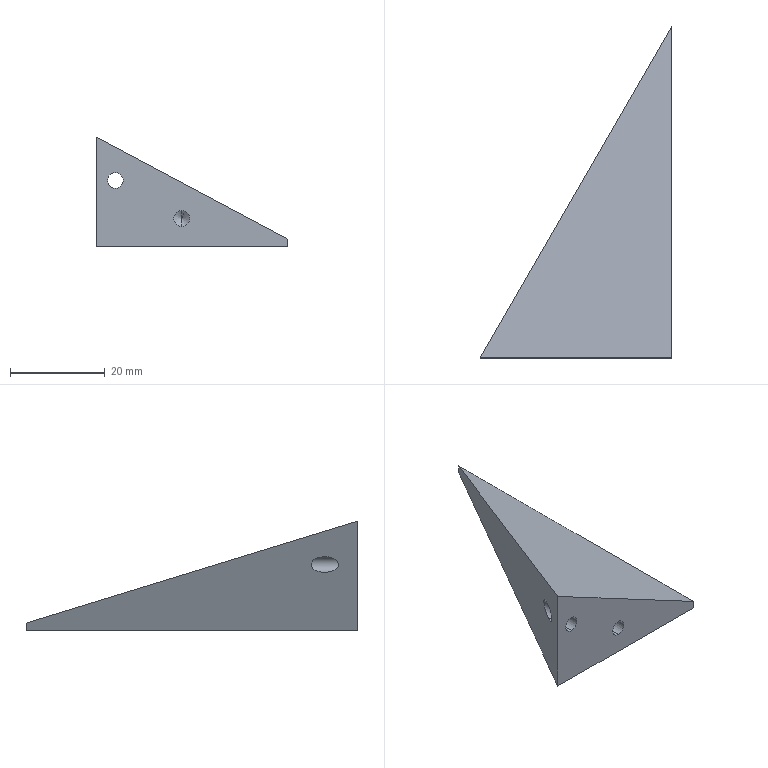Part | STEP file | GLSJ-10-26(2)_default | 1 solid | 11 faces | box 40.415 x 70 x 23.157 mm | volume 12326 mm3 | plane 5 | cylinder 4 | cone 2 | commonest cylinder face diameters 3.3 x4
STEP:
#1=CARTESIAN_POINT('',(0.,0.,0.));
#2=DIRECTION('',(0.,0.,1.));
#3=DIRECTION('',(1.,0.,0.));
#4=AXIS2_PLACEMENT_3D('',#1,#2,#3);
#5=CARTESIAN_POINT('',(-22.372,12.,-16.35));
#6=VERTEX_POINT('',#5);
#7=CARTESIAN_POINT('',(-22.372,12.,-19.65));
#8=VERTEX_POINT('',#7);
#9=CARTESIAN_POINT('',(-22.372,12.,-18.));
#10=DIRECTION('',(0.,-1.,0.));
#11=DIRECTION('',(0.,0.,-1.));
#12=AXIS2_PLACEMENT_3D('',#9,#10,#11);
#13=CIRCLE('',#12,1.65);
#14=CARTESIAN_POINT('',(-22.372,12.,-18.));
#15=DIRECTION('',(0.,-1.,0.));
#16=DIRECTION('',(0.,0.,-1.));
#17=AXIS2_PLACEMENT_3D('',#14,#15,#16);
#18=CONICAL_SURFACE('',#17,1.65,1.03);
#19=CARTESIAN_POINT('',(0.,0.));
#20=DIRECTION('',(1.,0.));
#21=VECTOR('',#20,1.);
#22=LINE('',#19,#21);
#23=(GEOMETRIC_REPRESENTATION_CONTEXT(2)PARAMETRIC_REPRESENTATION_CONTEXT()REPRESENTATION_CONTEXT('',''));
#24=DEFINITIONAL_REPRESENTATION('',(#22),#23);
#25=PCURVE('',#18,#24);
#26=CARTESIAN_POINT('',(-22.372,0.,-18.));
#27=DIRECTION('',(0.,-1.,0.));
#28=DIRECTION('',(0.,0.,1.));
#29=AXIS2_PLACEMENT_3D('',#26,#27,#28);
#30=CYLINDRICAL_SURFACE('',#29,1.65);
#31=CARTESIAN_POINT('',(-3.142,-12.));
#32=DIRECTION('',(1.,0.));
#33=VECTOR('',#32,1.);
#34=LINE('',#31,#33);
#35=(GEOMETRIC_REPRESENTATION_CONTEXT(2)PARAMETRIC_REPRESENTATION_CONTEXT()REPRESENTATION_CONTEXT('',''));
#36=DEFINITIONAL_REPRESENTATION('',(#34),#35);
#37=PCURVE('',#30,#36);
#38=SURFACE_CURVE('',#13,(#25,#37),.PCURVE_S1.);
#39=EDGE_CURVE('',#6,#8,#38,.T.);
#40=ORIENTED_EDGE('',*,*,#39,.F.);
#41=CARTESIAN_POINT('',(-22.372,12.991,-18.));
#42=VERTEX_POINT('',#41);
#43=CARTESIAN_POINT('',(-22.372,12.,-16.35));
#44=DIRECTION('',(0.,-0.515,0.8572));
#45=VECTOR('',#44,1.);
#46=LINE('',#43,#45);
#47=CARTESIAN_POINT('',(3.142,-0.9914));
#48=CARTESIAN_POINT('',(3.142,-0.9764));
#49=CARTESIAN_POINT('',(3.142,-0.9464));
#50=CARTESIAN_POINT('',(3.142,-0.9013));
#51=CARTESIAN_POINT('',(3.142,-0.8562));
#52=CARTESIAN_POINT('',(3.142,-0.8112));
#53=CARTESIAN_POINT('',(3.142,-0.7661));
#54=CARTESIAN_POINT('',(3.142,-0.721));
#55=CARTESIAN_POINT('',(3.142,-0.676));
#56=CARTESIAN_POINT('',(3.142,-0.6309));
#57=CARTESIAN_POINT('',(3.142,-0.5858));
#58=CARTESIAN_POINT('',(3.142,-0.5408));
#59=CARTESIAN_POINT('',(3.142,-0.4957));
#60=CARTESIAN_POINT('',(3.142,-0.4506));
#61=CARTESIAN_POINT('',(3.142,-0.4056));
#62=CARTESIAN_POINT('',(3.142,-0.3605));
#63=CARTESIAN_POINT('',(3.142,-0.3155));
#64=CARTESIAN_POINT('',(3.142,-0.2704));
#65=CARTESIAN_POINT('',(3.142,-0.2253));
#66=CARTESIAN_POINT('',(3.142,-0.1803));
#67=CARTESIAN_POINT('',(3.142,-0.1352));
#68=CARTESIAN_POINT('',(3.142,-0.09013));
#69=CARTESIAN_POINT('',(3.142,-0.04506));
#70=CARTESIAN_POINT('',(3.142,-0.01502));
#71=CARTESIAN_POINT('',(3.142,0.));
#72=B_SPLINE_CURVE_WITH_KNOTS('',3,(#47,#48,#49,#50,#51,#52,#53,#54,#55,#56,#57,#58,#59,#60,#61,#62,#63,#64,#65,#66,#67,#68,#69,#70,#71),.UNSPECIFIED.,.F.,.F.,(4,1,1,1,1,1,1,1,1,1,1,1,1,1,1,1,1,1,1,1,1,1,4),(-1.925,-1.837,-1.75,-1.662,-1.575,-1.487,-1.4,-1.312,-1.225,-1.137,-1.05,-0.9625,-0.875,-0.7875,-0.7,-0.6125,-0.525,-0.4375,-0.35,-0.2625,-0.175,-0.0875,0.),.QUASI_UNIFORM_KNOTS.);
#73=(GEOMETRIC_REPRESENTATION_CONTEXT(2)PARAMETRIC_REPRESENTATION_CONTEXT()REPRESENTATION_CONTEXT('',''));
#74=DEFINITIONAL_REPRESENTATION('',(#72),#73);
#75=PCURVE('',#18,#74);
#76=CARTESIAN_POINT('',(-22.372,12.,-18.));
#77=DIRECTION('',(0.,-1.,0.));
#78=DIRECTION('',(0.,0.,-1.));
#79=AXIS2_PLACEMENT_3D('',#76,#77,#78);
#80=CONICAL_SURFACE('',#79,1.65,1.03);
#81=CARTESIAN_POINT('',(3.142,-0.9914));
#82=CARTESIAN_POINT('',(3.142,-0.9764));
#83=CARTESIAN_POINT('',(3.142,-0.9464));
#84=CARTESIAN_POINT('',(3.142,-0.9013));
#85=CARTESIAN_POINT('',(3.142,-0.8562));
#86=CARTESIAN_POINT('',(3.142,-0.8112));
#87=CARTESIAN_POINT('',(3.142,-0.7661));
#88=CARTESIAN_POINT('',(3.142,-0.721));
#89=CARTESIAN_POINT('',(3.142,-0.676));
#90=CARTESIAN_POINT('',(3.142,-0.6309));
#91=CARTESIAN_POINT('',(3.142,-0.5858));
#92=CARTESIAN_POINT('',(3.142,-0.5408));
#93=CARTESIAN_POINT('',(3.142,-0.4957));
#94=CARTESIAN_POINT('',(3.142,-0.4506));
#95=CARTESIAN_POINT('',(3.142,-0.4056));
#96=CARTESIAN_POINT('',(3.142,-0.3605));
#97=CARTESIAN_POINT('',(3.142,-0.3155));
#98=CARTESIAN_POINT('',(3.142,-0.2704));
#99=CARTESIAN_POINT('',(3.142,-0.2253));
#100=CARTESIAN_POINT('',(3.142,-0.1803));
#101=CARTESIAN_POINT('',(3.142,-0.1352));
#102=CARTESIAN_POINT('',(3.142,-0.09013));
#103=CARTESIAN_POINT('',(3.142,-0.04506));
#104=CARTESIAN_POINT('',(3.142,-0.01502));
#105=CARTESIAN_POINT('',(3.142,0.));
#106=B_SPLINE_CURVE_WITH_KNOTS('',3,(#81,#82,#83,#84,#85,#86,#87,#88,#89,#90,#91,#92,#93,#94,#95,#96,#97,#98,#99,#100,#101,#102,#103,#104,#105),.UNSPECIFIED.,.F.,.F.,(4,1,1,1,1,1,1,1,1,1,1,1,1,1,1,1,1,1,1,1,1,1,4),(-1.925,-1.837,-1.75,-1.662,-1.575,-1.487,-1.4,-1.312,-1.225,-1.137,-1.05,-0.9625,-0.875,-0.7875,-0.7,-0.6125,-0.525,-0.4375,-0.35,-0.2625,-0.175,-0.0875,0.),.QUASI_UNIFORM_KNOTS.);
#107=(GEOMETRIC_REPRESENTATION_CONTEXT(2)PARAMETRIC_REPRESENTATION_CONTEXT()REPRESENTATION_CONTEXT('',''));
#108=DEFINITIONAL_REPRESENTATION('',(#106),#107);
#109=PCURVE('',#80,#108);
#110=SURFACE_CURVE('',#46,(#75,#109),.PCURVE_S1.);
#111=EDGE_CURVE('',#42,#6,#110,.T.);
#112=ORIENTED_EDGE('',*,*,#111,.F.);
#113=CARTESIAN_POINT('',(-22.372,12.,-19.65));
#114=DIRECTION('',(0.,-0.515,-0.8572));
#115=VECTOR('',#114,1.);
#116=LINE('',#113,#115);
#117=CARTESIAN_POINT('',(6.283,0.));
#118=DIRECTION('',(0.,1.));
#119=VECTOR('',#118,1.);
#120=LINE('',#117,#119);
#121=(GEOMETRIC_REPRESENTATION_CONTEXT(2)PARAMETRIC_REPRESENTATION_CONTEXT()REPRESENTATION_CONTEXT('',''));
#122=DEFINITIONAL_REPRESENTATION('',(#120),#121);
#123=PCURVE('',#18,#122);
#124=CARTESIAN_POINT('',(0.,0.));
#125=DIRECTION('',(0.,1.));
#126=VECTOR('',#125,1.);
#127=LINE('',#124,#126);
#128=(GEOMETRIC_REPRESENTATION_CONTEXT(2)PARAMETRIC_REPRESENTATION_CONTEXT()REPRESENTATION_CONTEXT('',''));
#129=DEFINITIONAL_REPRESENTATION('',(#127),#128);
#130=PCURVE('',#80,#129);
#131=SURFACE_CURVE('',#116,(#123,#130),.PCURVE_S1.);
#132=EDGE_CURVE('',#42,#8,#131,.T.);
#133=ORIENTED_EDGE('',*,*,#132,.T.);
#134=EDGE_LOOP('',(#40,#112,#133));
#135=FACE_BOUND('',#134,.F.);
#136=ADVANCED_FACE('',(#135),#18,.F.);
#137=CARTESIAN_POINT('',(-36.372,7.003,-8.35));
#138=VERTEX_POINT('',#137);
#139=CARTESIAN_POINT('',(-36.372,0.,-8.35));
#140=VERTEX_POINT('',#139);
#141=CARTESIAN_POINT('',(-36.372,0.,-8.35));
#142=DIRECTION('',(0.,-1.,0.));
#143=VECTOR('',#142,1.);
#144=LINE('',#141,#143);
#145=CARTESIAN_POINT('',(-36.372,0.,-10.));
#146=DIRECTION('',(0.,-1.,0.));
#147=DIRECTION('',(0.,0.,1.));
#148=AXIS2_PLACEMENT_3D('',#145,#146,#147);
#149=CYLINDRICAL_SURFACE('',#148,1.65);
#150=CARTESIAN_POINT('',(6.283,0.));
#151=DIRECTION('',(0.,1.));
#152=VECTOR('',#151,1.);
#153=LINE('',#150,#152);
#154=(GEOMETRIC_REPRESENTATION_CONTEXT(2)PARAMETRIC_REPRESENTATION_CONTEXT()REPRESENTATION_CONTEXT('',''));
#155=DEFINITIONAL_REPRESENTATION('',(#153),#154);
#156=PCURVE('',#149,#155);
#157=CARTESIAN_POINT('',(-36.372,0.,-10.));
#158=DIRECTION('',(0.,-1.,0.));
#159=DIRECTION('',(0.,0.,1.));
#160=AXIS2_PLACEMENT_3D('',#157,#158,#159);
#161=CYLINDRICAL_SURFACE('',#160,1.65);
#162=CARTESIAN_POINT('',(0.,0.));
#163=DIRECTION('',(0.,1.));
#164=VECTOR('',#163,1.);
#165=LINE('',#162,#164);
#166=(GEOMETRIC_REPRESENTATION_CONTEXT(2)PARAMETRIC_REPRESENTATION_CONTEXT()REPRESENTATION_CONTEXT('',''));
#167=DEFINITIONAL_REPRESENTATION('',(#165),#166);
#168=PCURVE('',#161,#167);
#169=SURFACE_CURVE('',#144,(#156,#168),.PCURVE_S1.);
#170=EDGE_CURVE('',#138,#140,#169,.T.);
#171=ORIENTED_EDGE('',*,*,#170,.T.);
#172=CARTESIAN_POINT('',(-36.372,0.,-11.65));
#173=VERTEX_POINT('',#172);
#174=CARTESIAN_POINT('',(-36.372,0.,-10.));
#175=DIRECTION('',(0.,1.,0.));
#176=DIRECTION('',(0.,0.,1.));
#177=AXIS2_PLACEMENT_3D('',#174,#175,#176);
#178=CIRCLE('',#177,1.65);
#179=CARTESIAN_POINT('',(6.283,0.));
#180=DIRECTION('',(-1.,0.));
#181=VECTOR('',#180,1.);
#182=LINE('',#179,#181);
#183=(GEOMETRIC_REPRESENTATION_CONTEXT(2)PARAMETRIC_REPRESENTATION_CONTEXT()REPRESENTATION_CONTEXT('',''));
#184=DEFINITIONAL_REPRESENTATION('',(#182),#183);
#185=PCURVE('',#149,#184);
#186=CARTESIAN_POINT('',(-40.415,0.,-24.));
#187=DIRECTION('',(0.,1.,0.));
#188=DIRECTION('',(-1.,0.,0.));
#189=AXIS2_PLACEMENT_3D('',#186,#187,#188);
#190=PLANE('',#189);
#191=CARTESIAN_POINT('',(-4.043,14.));
#192=DIRECTION('',(0.,1.));
#193=AXIS2_PLACEMENT_2D('',#191,#192);
#194=CIRCLE('',#193,1.65);
#195=(GEOMETRIC_REPRESENTATION_CONTEXT(2)PARAMETRIC_REPRESENTATION_CONTEXT()REPRESENTATION_CONTEXT('',''));
#196=DEFINITIONAL_REPRESENTATION('',(#194),#195);
#197=PCURVE('',#190,#196);
#198=SURFACE_CURVE('',#178,(#185,#197),.PCURVE_S1.);
#199=EDGE_CURVE('',#140,#173,#198,.T.);
#200=ORIENTED_EDGE('',*,*,#199,.T.);
#201=CARTESIAN_POINT('',(-36.372,7.003,-11.65));
#202=VERTEX_POINT('',#201);
#203=CARTESIAN_POINT('',(-36.372,0.,-11.65));
#204=DIRECTION('',(0.,-1.,0.));
#205=VECTOR('',#204,1.);
#206=LINE('',#203,#205);
#207=CARTESIAN_POINT('',(3.142,0.));
#208=DIRECTION('',(0.,1.));
#209=VECTOR('',#208,1.);
#210=LINE('',#207,#209);
#211=(GEOMETRIC_REPRESENTATION_CONTEXT(2)PARAMETRIC_REPRESENTATION_CONTEXT()REPRESENTATION_CONTEXT('',''));
#212=DEFINITIONAL_REPRESENTATION('',(#210),#211);
#213=PCURVE('',#149,#212);
#214=CARTESIAN_POINT('',(3.142,0.));
#215=DIRECTION('',(0.,1.));
#216=VECTOR('',#215,1.);
#217=LINE('',#214,#216);
#218=(GEOMETRIC_REPRESENTATION_CONTEXT(2)PARAMETRIC_REPRESENTATION_CONTEXT()REPRESENTATION_CONTEXT('',''));
#219=DEFINITIONAL_REPRESENTATION('',(#217),#218);
#220=PCURVE('',#161,#219);
#221=SURFACE_CURVE('',#206,(#213,#220),.PCURVE_S1.);
#222=EDGE_CURVE('',#202,#173,#221,.T.);
#223=ORIENTED_EDGE('',*,*,#222,.F.);
#224=CARTESIAN_POINT('',(-36.372,7.003,-8.35));
#225=CARTESIAN_POINT('',(-33.072,12.718,-8.35));
#226=CARTESIAN_POINT('',(-33.072,12.718,-11.65));
#227=CARTESIAN_POINT('',(-36.372,7.003,-11.65));
#228=(BOUNDED_CURVE()B_SPLINE_CURVE(3,(#224,#225,#226,#227),.UNSPECIFIED.,.F.,.F.)B_SPLINE_CURVE_WITH_KNOTS((4,4),(1.571,4.712),.PIECEWISE_BEZIER_KNOTS.)CURVE()GEOMETRIC_REPRESENTATION_ITEM()RATIONAL_B_SPLINE_CURVE((1.,0.3333,0.3333,1.))REPRESENTATION_ITEM(''));
#229=CARTESIAN_POINT('',(6.283,-7.003));
#230=CARTESIAN_POINT('',(6.253,-7.089));
#231=CARTESIAN_POINT('',(6.19,-7.27));
#232=CARTESIAN_POINT('',(6.085,-7.565));
#233=CARTESIAN_POINT('',(5.972,-7.88));
#234=CARTESIAN_POINT('',(5.848,-8.212));
#235=CARTESIAN_POINT('',(5.713,-8.551));
#236=CARTESIAN_POINT('',(5.567,-8.885));
#237=CARTESIAN_POINT('',(5.412,-9.199));
#238=CARTESIAN_POINT('',(5.246,-9.475));
#239=CARTESIAN_POINT('',(5.073,-9.69));
#240=CARTESIAN_POINT('',(4.894,-9.829));
#241=CARTESIAN_POINT('',(4.712,-9.876));
#242=CARTESIAN_POINT('',(4.531,-9.829));
#243=CARTESIAN_POINT('',(4.352,-9.69));
#244=CARTESIAN_POINT('',(4.179,-9.475));
#245=CARTESIAN_POINT('',(4.013,-9.199));
#246=CARTESIAN_POINT('',(3.857,-8.885));
#247=CARTESIAN_POINT('',(3.712,-8.551));
#248=CARTESIAN_POINT('',(3.577,-8.212));
#249=CARTESIAN_POINT('',(3.453,-7.88));
#250=CARTESIAN_POINT('',(3.339,-7.565));
#251=CARTESIAN_POINT('',(3.235,-7.27));
#252=CARTESIAN_POINT('',(3.172,-7.089));
#253=CARTESIAN_POINT('',(3.142,-7.003));
#254=B_SPLINE_CURVE_WITH_KNOTS('',3,(#229,#230,#231,#232,#233,#234,#235,#236,#237,#238,#239,#240,#241,#242,#243,#244,#245,#246,#247,#248,#249,#250,#251,#252,#253),.UNSPECIFIED.,.F.,.F.,(4,1,1,1,1,1,1,1,1,1,1,1,1,1,1,1,1,1,1,1,1,1,4),(1.571,1.714,1.856,1.999,2.142,2.285,2.428,2.57,2.713,2.856,2.999,3.142,3.284,3.427,3.57,3.713,3.856,3.998,4.141,4.284,4.427,4.57,4.712),.QUASI_UNIFORM_KNOTS.);
#255=(GEOMETRIC_REPRESENTATION_CONTEXT(2)PARAMETRIC_REPRESENTATION_CONTEXT()REPRESENTATION_CONTEXT('',''));
#256=DEFINITIONAL_REPRESENTATION('',(#254),#255);
#257=PCURVE('',#149,#256);
#258=CARTESIAN_POINT('',(0.,70.,-24.));
#259=DIRECTION('',(0.866,-0.5,0.));
#260=DIRECTION('',(0.5,0.866,0.));
#261=AXIS2_PLACEMENT_3D('',#258,#259,#260);
#262=PLANE('',#261);
#263=CARTESIAN_POINT('',(-72.743,15.65));
#264=CARTESIAN_POINT('',(-66.143,15.65));
#265=CARTESIAN_POINT('',(-66.143,12.35));
#266=CARTESIAN_POINT('',(-72.743,12.35));
#267=(BOUNDED_CURVE()B_SPLINE_CURVE(3,(#263,#264,#265,#266),.UNSPECIFIED.,.F.,.F.)B_SPLINE_CURVE_WITH_KNOTS((4,4),(1.571,4.712),.PIECEWISE_BEZIER_KNOTS.)CURVE()GEOMETRIC_REPRESENTATION_ITEM()RATIONAL_B_SPLINE_CURVE((1.,0.3333,0.3333,1.))REPRESENTATION_ITEM(''));
#268=(GEOMETRIC_REPRESENTATION_CONTEXT(2)PARAMETRIC_REPRESENTATION_CONTEXT()REPRESENTATION_CONTEXT('',''));
#269=DEFINITIONAL_REPRESENTATION('',(#267),#268);
#270=PCURVE('',#262,#269);
#271=SURFACE_CURVE('',#228,(#257,#270),.PCURVE_S1.);
#272=EDGE_CURVE('',#138,#202,#271,.T.);
#273=ORIENTED_EDGE('',*,*,#272,.F.);
#274=EDGE_LOOP('',(#171,#200,#223,#273));
#275=FACE_BOUND('',#274,.F.);
#276=ADVANCED_FACE('',(#275),#149,.F.);
#277=CARTESIAN_POINT('',(-22.372,0.,-16.35));
#278=VERTEX_POINT('',#277);
#279=CARTESIAN_POINT('',(-22.372,0.,-16.35));
#280=DIRECTION('',(0.,-1.,0.));
#281=VECTOR('',#280,1.);
#282=LINE('',#279,#281);
#283=CARTESIAN_POINT('',(-22.372,0.,-18.));
#284=DIRECTION('',(0.,-1.,0.));
#285=DIRECTION('',(0.,0.,1.));
#286=AXIS2_PLACEMENT_3D('',#283,#284,#285);
#287=CYLINDRICAL_SURFACE('',#286,1.65);
#288=CARTESIAN_POINT('',(6.283,0.));
#289=DIRECTION('',(0.,1.));
#290=VECTOR('',#289,1.);
#291=LINE('',#288,#290);
#292=(GEOMETRIC_REPRESENTATION_CONTEXT(2)PARAMETRIC_REPRESENTATION_CONTEXT()REPRESENTATION_CONTEXT('',''));
#293=DEFINITIONAL_REPRESENTATION('',(#291),#292);
#294=PCURVE('',#287,#293);
#295=CARTESIAN_POINT('',(0.,0.));
#296=DIRECTION('',(0.,1.));
#297=VECTOR('',#296,1.);
#298=LINE('',#295,#297);
#299=(GEOMETRIC_REPRESENTATION_CONTEXT(2)PARAMETRIC_REPRESENTATION_CONTEXT()REPRESENTATION_CONTEXT('',''));
#300=DEFINITIONAL_REPRESENTATION('',(#298),#299);
#301=PCURVE('',#30,#300);
#302=SURFACE_CURVE('',#282,(#294,#301),.PCURVE_S1.);
#303=EDGE_CURVE('',#6,#278,#302,.T.);
#304=ORIENTED_EDGE('',*,*,#303,.T.);
#305=CARTESIAN_POINT('',(-22.372,0.,-19.65));
#306=VERTEX_POINT('',#305);
#307=CARTESIAN_POINT('',(-22.372,0.,-18.));
#308=DIRECTION('',(0.,1.,0.));
#309=DIRECTION('',(0.,0.,1.));
#310=AXIS2_PLACEMENT_3D('',#307,#308,#309);
#311=CIRCLE('',#310,1.65);
#312=CARTESIAN_POINT('',(6.283,0.));
#313=DIRECTION('',(-1.,0.));
#314=VECTOR('',#313,1.);
#315=LINE('',#312,#314);
#316=(GEOMETRIC_REPRESENTATION_CONTEXT(2)PARAMETRIC_REPRESENTATION_CONTEXT()REPRESENTATION_CONTEXT('',''));
#317=DEFINITIONAL_REPRESENTATION('',(#315),#316);
#318=PCURVE('',#287,#317);
#319=CARTESIAN_POINT('',(-18.043,6.));
#320=DIRECTION('',(0.,1.));
#321=AXIS2_PLACEMENT_2D('',#319,#320);
#322=CIRCLE('',#321,1.65);
#323=(GEOMETRIC_REPRESENTATION_CONTEXT(2)PARAMETRIC_REPRESENTATION_CONTEXT()REPRESENTATION_CONTEXT('',''));
#324=DEFINITIONAL_REPRESENTATION('',(#322),#323);
#325=PCURVE('',#190,#324);
#326=SURFACE_CURVE('',#311,(#318,#325),.PCURVE_S1.);
#327=EDGE_CURVE('',#278,#306,#326,.T.);
#328=ORIENTED_EDGE('',*,*,#327,.T.);
#329=CARTESIAN_POINT('',(-22.372,0.,-19.65));
#330=DIRECTION('',(0.,-1.,0.));
#331=VECTOR('',#330,1.);
#332=LINE('',#329,#331);
#333=CARTESIAN_POINT('',(3.142,0.));
#334=DIRECTION('',(0.,1.));
#335=VECTOR('',#334,1.);
#336=LINE('',#333,#335);
#337=(GEOMETRIC_REPRESENTATION_CONTEXT(2)PARAMETRIC_REPRESENTATION_CONTEXT()REPRESENTATION_CONTEXT('',''));
#338=DEFINITIONAL_REPRESENTATION('',(#336),#337);
#339=PCURVE('',#287,#338);
#340=CARTESIAN_POINT('',(3.142,0.));
#341=DIRECTION('',(0.,1.));
#342=VECTOR('',#341,1.);
#343=LINE('',#340,#342);
#344=(GEOMETRIC_REPRESENTATION_CONTEXT(2)PARAMETRIC_REPRESENTATION_CONTEXT()REPRESENTATION_CONTEXT('',''));
#345=DEFINITIONAL_REPRESENTATION('',(#343),#344);
#346=PCURVE('',#30,#345);
#347=SURFACE_CURVE('',#332,(#339,#346),.PCURVE_S1.);
#348=EDGE_CURVE('',#8,#306,#347,.T.);
#349=ORIENTED_EDGE('',*,*,#348,.F.);
#350=CARTESIAN_POINT('',(-22.372,12.,-18.));
#351=DIRECTION('',(0.,-1.,0.));
#352=DIRECTION('',(0.,0.,-1.));
#353=AXIS2_PLACEMENT_3D('',#350,#351,#352);
#354=CIRCLE('',#353,1.65);
#355=CARTESIAN_POINT('',(3.142,-12.));
#356=DIRECTION('',(1.,0.));
#357=VECTOR('',#356,1.);
#358=LINE('',#355,#357);
#359=(GEOMETRIC_REPRESENTATION_CONTEXT(2)PARAMETRIC_REPRESENTATION_CONTEXT()REPRESENTATION_CONTEXT('',''));
#360=DEFINITIONAL_REPRESENTATION('',(#358),#359);
#361=PCURVE('',#287,#360);
#362=CARTESIAN_POINT('',(0.,0.));
#363=DIRECTION('',(1.,0.));
#364=VECTOR('',#363,1.);
#365=LINE('',#362,#364);
#366=(GEOMETRIC_REPRESENTATION_CONTEXT(2)PARAMETRIC_REPRESENTATION_CONTEXT()REPRESENTATION_CONTEXT('',''));
#367=DEFINITIONAL_REPRESENTATION('',(#365),#366);
#368=PCURVE('',#80,#367);
#369=SURFACE_CURVE('',#354,(#361,#368),.PCURVE_S1.);
#370=EDGE_CURVE('',#8,#6,#369,.T.);
#371=ORIENTED_EDGE('',*,*,#370,.T.);
#372=EDGE_LOOP('',(#304,#328,#349,#371));
#373=FACE_BOUND('',#372,.F.);
#374=ADVANCED_FACE('',(#373),#287,.F.);
#375=ORIENTED_EDGE('',*,*,#199,.T.);
#376=CARTESIAN_POINT('',(-36.372,0.,-10.));
#377=DIRECTION('',(0.,1.,0.));
#378=DIRECTION('',(0.,0.,1.));
#379=AXIS2_PLACEMENT_3D('',#376,#377,#378);
#380=CIRCLE('',#379,1.65);
#381=CARTESIAN_POINT('',(-4.043,14.));
#382=DIRECTION('',(0.,1.));
#383=AXIS2_PLACEMENT_2D('',#381,#382);
#384=CIRCLE('',#383,1.65);
#385=(GEOMETRIC_REPRESENTATION_CONTEXT(2)PARAMETRIC_REPRESENTATION_CONTEXT()REPRESENTATION_CONTEXT('',''));
#386=DEFINITIONAL_REPRESENTATION('',(#384),#385);
#387=PCURVE('',#190,#386);
#388=CARTESIAN_POINT('',(6.283,0.));
#389=DIRECTION('',(-1.,0.));
#390=VECTOR('',#389,1.);
#391=LINE('',#388,#390);
#392=(GEOMETRIC_REPRESENTATION_CONTEXT(2)PARAMETRIC_REPRESENTATION_CONTEXT()REPRESENTATION_CONTEXT('',''));
#393=DEFINITIONAL_REPRESENTATION('',(#391),#392);
#394=PCURVE('',#161,#393);
#395=SURFACE_CURVE('',#380,(#387,#394),.PCURVE_S1.);
#396=EDGE_CURVE('',#173,#140,#395,.T.);
#397=ORIENTED_EDGE('',*,*,#396,.T.);
#398=EDGE_LOOP('',(#375,#397));
#399=FACE_BOUND('',#398,.T.);
#400=ORIENTED_EDGE('',*,*,#327,.T.);
#401=CARTESIAN_POINT('',(-22.372,0.,-18.));
#402=DIRECTION('',(0.,1.,0.));
#403=DIRECTION('',(0.,0.,1.));
#404=AXIS2_PLACEMENT_3D('',#401,#402,#403);
#405=CIRCLE('',#404,1.65);
#406=CARTESIAN_POINT('',(-18.043,6.));
#407=DIRECTION('',(0.,1.));
#408=AXIS2_PLACEMENT_2D('',#406,#407);
#409=CIRCLE('',#408,1.65);
#410=(GEOMETRIC_REPRESENTATION_CONTEXT(2)PARAMETRIC_REPRESENTATION_CONTEXT()REPRESENTATION_CONTEXT('',''));
#411=DEFINITIONAL_REPRESENTATION('',(#409),#410);
#412=PCURVE('',#190,#411);
#413=CARTESIAN_POINT('',(6.283,0.));
#414=DIRECTION('',(-1.,0.));
#415=VECTOR('',#414,1.);
#416=LINE('',#413,#415);
#417=(GEOMETRIC_REPRESENTATION_CONTEXT(2)PARAMETRIC_REPRESENTATION_CONTEXT()REPRESENTATION_CONTEXT('',''));
#418=DEFINITIONAL_REPRESENTATION('',(#416),#417);
#419=PCURVE('',#30,#418);
#420=SURFACE_CURVE('',#405,(#412,#419),.PCURVE_S1.);
#421=EDGE_CURVE('',#306,#278,#420,.T.);
#422=ORIENTED_EDGE('',*,*,#421,.T.);
#423=EDGE_LOOP('',(#400,#422));
#424=FACE_BOUND('',#423,.T.);
#425=CARTESIAN_POINT('',(-40.415,0.,-24.));
#426=VERTEX_POINT('',#425);
#427=CARTESIAN_POINT('',(-40.415,0.,-0.843));
#428=VERTEX_POINT('',#427);
#429=CARTESIAN_POINT('',(-40.415,0.,-24.));
#430=DIRECTION('',(0.,0.,1.));
#431=VECTOR('',#430,1.);
#432=LINE('',#429,#431);
#433=CARTESIAN_POINT('',(0.,0.));
#434=DIRECTION('',(0.,1.));
#435=VECTOR('',#434,1.);
#436=LINE('',#433,#435);
#437=(GEOMETRIC_REPRESENTATION_CONTEXT(2)PARAMETRIC_REPRESENTATION_CONTEXT()REPRESENTATION_CONTEXT('',''));
#438=DEFINITIONAL_REPRESENTATION('',(#436),#437);
#439=PCURVE('',#190,#438);
#440=CARTESIAN_POINT('',(-80.829,0.));
#441=DIRECTION('',(0.,1.));
#442=VECTOR('',#441,1.);
#443=LINE('',#440,#442);
#444=(GEOMETRIC_REPRESENTATION_CONTEXT(2)PARAMETRIC_REPRESENTATION_CONTEXT()REPRESENTATION_CONTEXT('',''));
#445=DEFINITIONAL_REPRESENTATION('',(#443),#444);
#446=PCURVE('',#262,#445);
#447=SURFACE_CURVE('',#432,(#439,#446),.PCURVE_S1.);
#448=EDGE_CURVE('',#426,#428,#447,.T.);
#449=ORIENTED_EDGE('',*,*,#448,.F.);
#450=CARTESIAN_POINT('',(0.,0.,-24.));
#451=VERTEX_POINT('',#450);
#452=CARTESIAN_POINT('',(-40.415,0.,-24.));
#453=DIRECTION('',(1.,0.,0.));
#454=VECTOR('',#453,1.);
#455=LINE('',#452,#454);
#456=CARTESIAN_POINT('',(0.,0.));
#457=DIRECTION('',(-1.,0.));
#458=VECTOR('',#457,1.);
#459=LINE('',#456,#458);
#460=(GEOMETRIC_REPRESENTATION_CONTEXT(2)PARAMETRIC_REPRESENTATION_CONTEXT()REPRESENTATION_CONTEXT('',''));
#461=DEFINITIONAL_REPRESENTATION('',(#459),#460);
#462=PCURVE('',#190,#461);
#463=CARTESIAN_POINT('',(0.,0.,-24.));
#464=DIRECTION('',(0.,0.,-1.));
#465=DIRECTION('',(1.,0.,0.));
#466=AXIS2_PLACEMENT_3D('',#463,#464,#465);
#467=PLANE('',#466);
#468=CARTESIAN_POINT('',(-40.415,0.));
#469=DIRECTION('',(1.,0.));
#470=VECTOR('',#469,1.);
#471=LINE('',#468,#470);
#472=(GEOMETRIC_REPRESENTATION_CONTEXT(2)PARAMETRIC_REPRESENTATION_CONTEXT()REPRESENTATION_CONTEXT('',''));
#473=DEFINITIONAL_REPRESENTATION('',(#471),#472);
#474=PCURVE('',#467,#473);
#475=SURFACE_CURVE('',#455,(#462,#474),.PCURVE_S1.);
#476=EDGE_CURVE('',#426,#451,#475,.T.);
#477=ORIENTED_EDGE('',*,*,#476,.T.);
#478=CARTESIAN_POINT('',(0.,0.,-22.332));
#479=VERTEX_POINT('',#478);
#480=CARTESIAN_POINT('',(0.,0.,-24.));
#481=DIRECTION('',(0.,0.,1.));
#482=VECTOR('',#481,1.);
#483=LINE('',#480,#482);
#484=CARTESIAN_POINT('',(-40.415,0.));
#485=DIRECTION('',(0.,1.));
#486=VECTOR('',#485,1.);
#487=LINE('',#484,#486);
#488=(GEOMETRIC_REPRESENTATION_CONTEXT(2)PARAMETRIC_REPRESENTATION_CONTEXT()REPRESENTATION_CONTEXT('',''));
#489=DEFINITIONAL_REPRESENTATION('',(#487),#488);
#490=PCURVE('',#190,#489);
#491=CARTESIAN_POINT('',(0.,0.,-24.));
#492=DIRECTION('',(-1.,0.,0.));
#493=DIRECTION('',(0.,0.,-1.));
#494=AXIS2_PLACEMENT_3D('',#491,#492,#493);
#495=PLANE('',#494);
#496=CARTESIAN_POINT('',(0.,0.));
#497=DIRECTION('',(-1.,0.));
#498=VECTOR('',#497,1.);
#499=LINE('',#496,#498);
#500=(GEOMETRIC_REPRESENTATION_CONTEXT(2)PARAMETRIC_REPRESENTATION_CONTEXT()REPRESENTATION_CONTEXT('',''));
#501=DEFINITIONAL_REPRESENTATION('',(#499),#500);
#502=PCURVE('',#495,#501);
#503=SURFACE_CURVE('',#483,(#490,#502),.PCURVE_S1.);
#504=EDGE_CURVE('',#451,#479,#503,.T.);
#505=ORIENTED_EDGE('',*,*,#504,.T.);
#506=CARTESIAN_POINT('',(0.,0.,-22.332));
#507=DIRECTION('',(0.8829,0.,-0.4695));
#508=VECTOR('',#507,1.);
#509=LINE('',#506,#508);
#510=CARTESIAN_POINT('',(-40.415,1.668));
#511=DIRECTION('',(-0.8829,-0.4695));
#512=VECTOR('',#511,1.);
#513=LINE('',#510,#512);
#514=(GEOMETRIC_REPRESENTATION_CONTEXT(2)PARAMETRIC_REPRESENTATION_CONTEXT()REPRESENTATION_CONTEXT('',''));
#515=DEFINITIONAL_REPRESENTATION('',(#513),#514);
#516=PCURVE('',#190,#515);
#517=CARTESIAN_POINT('',(0.,0.,-22.332));
#518=DIRECTION('',(-0.4695,0.,-0.8829));
#519=DIRECTION('',(0.,1.,0.));
#520=AXIS2_PLACEMENT_3D('',#517,#518,#519);
#521=PLANE('',#520);
#522=CARTESIAN_POINT('',(0.,0.));
#523=DIRECTION('',(0.,1.));
#524=VECTOR('',#523,1.);
#525=LINE('',#522,#524);
#526=(GEOMETRIC_REPRESENTATION_CONTEXT(2)PARAMETRIC_REPRESENTATION_CONTEXT()REPRESENTATION_CONTEXT('',''));
#527=DEFINITIONAL_REPRESENTATION('',(#525),#526);
#528=PCURVE('',#521,#527);
#529=SURFACE_CURVE('',#509,(#516,#528),.PCURVE_S1.);
#530=EDGE_CURVE('',#428,#479,#529,.T.);
#531=ORIENTED_EDGE('',*,*,#530,.F.);
#532=EDGE_LOOP('',(#449,#477,#505,#531));
#533=FACE_BOUND('',#532,.T.);
#534=ADVANCED_FACE('',(#399,#424,#533),#190,.F.);
#535=ORIENTED_EDGE('',*,*,#504,.F.);
#536=CARTESIAN_POINT('',(0.,70.,-24.));
#537=VERTEX_POINT('',#536);
#538=CARTESIAN_POINT('',(0.,0.,-24.));
#539=DIRECTION('',(0.,1.,0.));
#540=VECTOR('',#539,1.);
#541=LINE('',#538,#540);
#542=CARTESIAN_POINT('',(0.,0.));
#543=DIRECTION('',(0.,-1.));
#544=VECTOR('',#543,1.);
#545=LINE('',#542,#544);
#546=(GEOMETRIC_REPRESENTATION_CONTEXT(2)PARAMETRIC_REPRESENTATION_CONTEXT()REPRESENTATION_CONTEXT('',''));
#547=DEFINITIONAL_REPRESENTATION('',(#545),#546);
#548=PCURVE('',#495,#547);
#549=CARTESIAN_POINT('',(0.,0.));
#550=DIRECTION('',(0.,-1.));
#551=VECTOR('',#550,1.);
#552=LINE('',#549,#551);
#553=(GEOMETRIC_REPRESENTATION_CONTEXT(2)PARAMETRIC_REPRESENTATION_CONTEXT()REPRESENTATION_CONTEXT('',''));
#554=DEFINITIONAL_REPRESENTATION('',(#552),#553);
#555=PCURVE('',#467,#554);
#556=SURFACE_CURVE('',#541,(#548,#555),.PCURVE_S1.);
#557=EDGE_CURVE('',#451,#537,#556,.T.);
#558=ORIENTED_EDGE('',*,*,#557,.T.);
#559=CARTESIAN_POINT('',(0.,70.,-22.332));
#560=VERTEX_POINT('',#559);
#561=CARTESIAN_POINT('',(0.,70.,-24.));
#562=DIRECTION('',(0.,0.,1.));
#563=VECTOR('',#562,1.);
#564=LINE('',#561,#563);
#565=CARTESIAN_POINT('',(0.,-70.));
#566=DIRECTION('',(-1.,0.));
#567=VECTOR('',#566,1.);
#568=LINE('',#565,#567);
#569=(GEOMETRIC_REPRESENTATION_CONTEXT(2)PARAMETRIC_REPRESENTATION_CONTEXT()REPRESENTATION_CONTEXT('',''));
#570=DEFINITIONAL_REPRESENTATION('',(#568),#569);
#571=PCURVE('',#495,#570);
#572=CARTESIAN_POINT('',(0.,0.));
#573=DIRECTION('',(0.,1.));
#574=VECTOR('',#573,1.);
#575=LINE('',#572,#574);
#576=(GEOMETRIC_REPRESENTATION_CONTEXT(2)PARAMETRIC_REPRESENTATION_CONTEXT()REPRESENTATION_CONTEXT('',''));
#577=DEFINITIONAL_REPRESENTATION('',(#575),#576);
#578=PCURVE('',#262,#577);
#579=SURFACE_CURVE('',#564,(#571,#578),.PCURVE_S1.);
#580=EDGE_CURVE('',#537,#560,#579,.T.);
#581=ORIENTED_EDGE('',*,*,#580,.T.);
#582=CARTESIAN_POINT('',(0.,0.,-22.332));
#583=DIRECTION('',(0.,1.,0.));
#584=VECTOR('',#583,1.);
#585=LINE('',#582,#584);
#586=CARTESIAN_POINT('',(-1.668,0.));
#587=DIRECTION('',(0.,-1.));
#588=VECTOR('',#587,1.);
#589=LINE('',#586,#588);
#590=(GEOMETRIC_REPRESENTATION_CONTEXT(2)PARAMETRIC_REPRESENTATION_CONTEXT()REPRESENTATION_CONTEXT('',''));
#591=DEFINITIONAL_REPRESENTATION('',(#589),#590);
#592=PCURVE('',#495,#591);
#593=CARTESIAN_POINT('',(0.,0.));
#594=DIRECTION('',(1.,0.));
#595=VECTOR('',#594,1.);
#596=LINE('',#593,#595);
#597=(GEOMETRIC_REPRESENTATION_CONTEXT(2)PARAMETRIC_REPRESENTATION_CONTEXT()REPRESENTATION_CONTEXT('',''));
#598=DEFINITIONAL_REPRESENTATION('',(#596),#597);
#599=PCURVE('',#521,#598);
#600=SURFACE_CURVE('',#585,(#592,#599),.PCURVE_S1.);
#601=EDGE_CURVE('',#479,#560,#600,.T.);
#602=ORIENTED_EDGE('',*,*,#601,.F.);
#603=EDGE_LOOP('',(#535,#558,#581,#602));
#604=FACE_BOUND('',#603,.T.);
#605=ADVANCED_FACE('',(#604),#495,.F.);
#606=ORIENTED_EDGE('',*,*,#272,.F.);
#607=CARTESIAN_POINT('',(-36.372,7.003,-11.65));
#608=CARTESIAN_POINT('',(-39.672,1.287,-11.65));
#609=CARTESIAN_POINT('',(-39.672,1.287,-8.35));
#610=CARTESIAN_POINT('',(-36.372,7.003,-8.35));
#611=(BOUNDED_CURVE()B_SPLINE_CURVE(3,(#607,#608,#609,#610),.UNSPECIFIED.,.F.,.F.)B_SPLINE_CURVE_WITH_KNOTS((4,4),(4.712,7.854),.PIECEWISE_BEZIER_KNOTS.)CURVE()GEOMETRIC_REPRESENTATION_ITEM()RATIONAL_B_SPLINE_CURVE((1.,0.3333,0.3333,1.))REPRESENTATION_ITEM(''));
#612=CARTESIAN_POINT('',(-72.743,12.35));
#613=CARTESIAN_POINT('',(-79.343,12.35));
#614=CARTESIAN_POINT('',(-79.343,15.65));
#615=CARTESIAN_POINT('',(-72.743,15.65));
#616=(BOUNDED_CURVE()B_SPLINE_CURVE(3,(#612,#613,#614,#615),.UNSPECIFIED.,.F.,.F.)B_SPLINE_CURVE_WITH_KNOTS((4,4),(4.712,7.854),.PIECEWISE_BEZIER_KNOTS.)CURVE()GEOMETRIC_REPRESENTATION_ITEM()RATIONAL_B_SPLINE_CURVE((1.,0.3333,0.3333,1.))REPRESENTATION_ITEM(''));
#617=(GEOMETRIC_REPRESENTATION_CONTEXT(2)PARAMETRIC_REPRESENTATION_CONTEXT()REPRESENTATION_CONTEXT('',''));
#618=DEFINITIONAL_REPRESENTATION('',(#616),#617);
#619=PCURVE('',#262,#618);
#620=CARTESIAN_POINT('',(3.142,-7.003));
#621=CARTESIAN_POINT('',(3.111,-6.916));
#622=CARTESIAN_POINT('',(3.048,-6.735));
#623=CARTESIAN_POINT('',(2.944,-6.44));
#624=CARTESIAN_POINT('',(2.83,-6.125));
#625=CARTESIAN_POINT('',(2.706,-5.793));
#626=CARTESIAN_POINT('',(2.571,-5.455));
#627=CARTESIAN_POINT('',(2.426,-5.12));
#628=CARTESIAN_POINT('',(2.27,-4.806));
#629=CARTESIAN_POINT('',(2.105,-4.531));
#630=CARTESIAN_POINT('',(1.931,-4.315));
#631=CARTESIAN_POINT('',(1.753,-4.176));
#632=CARTESIAN_POINT('',(1.571,-4.129));
#633=CARTESIAN_POINT('',(1.389,-4.176));
#634=CARTESIAN_POINT('',(1.21,-4.315));
#635=CARTESIAN_POINT('',(1.037,-4.531));
#636=CARTESIAN_POINT('',(0.8717,-4.806));
#637=CARTESIAN_POINT('',(0.7158,-5.12));
#638=CARTESIAN_POINT('',(0.5703,-5.455));
#639=CARTESIAN_POINT('',(0.4356,-5.793));
#640=CARTESIAN_POINT('',(0.3115,-6.125));
#641=CARTESIAN_POINT('',(0.1977,-6.44));
#642=CARTESIAN_POINT('',(0.09367,-6.735));
#643=CARTESIAN_POINT('',(0.0303,-6.916));
#644=CARTESIAN_POINT('',(0.,-7.003));
#645=B_SPLINE_CURVE_WITH_KNOTS('',3,(#620,#621,#622,#623,#624,#625,#626,#627,#628,#629,#630,#631,#632,#633,#634,#635,#636,#637,#638,#639,#640,#641,#642,#643,#644),.UNSPECIFIED.,.F.,.F.,(4,1,1,1,1,1,1,1,1,1,1,1,1,1,1,1,1,1,1,1,1,1,4),(4.712,4.855,4.998,5.141,5.284,5.426,5.569,5.712,5.855,5.998,6.14,6.283,6.426,6.569,6.712,6.854,6.997,7.14,7.283,7.426,7.568,7.711,7.854),.QUASI_UNIFORM_KNOTS.);
#646=(GEOMETRIC_REPRESENTATION_CONTEXT(2)PARAMETRIC_REPRESENTATION_CONTEXT()REPRESENTATION_CONTEXT('',''));
#647=DEFINITIONAL_REPRESENTATION('',(#645),#646);
#648=PCURVE('',#161,#647);
#649=SURFACE_CURVE('',#611,(#619,#648),.PCURVE_S1.);
#650=EDGE_CURVE('',#202,#138,#649,.T.);
#651=ORIENTED_EDGE('',*,*,#650,.F.);
#652=EDGE_LOOP('',(#606,#651));
#653=FACE_BOUND('',#652,.T.);
#654=ORIENTED_EDGE('',*,*,#580,.F.);
#655=CARTESIAN_POINT('',(0.,70.,-24.));
#656=DIRECTION('',(-0.5,-0.866,0.));
#657=VECTOR('',#656,1.);
#658=LINE('',#655,#657);
#659=CARTESIAN_POINT('',(0.,0.));
#660=DIRECTION('',(-1.,0.));
#661=VECTOR('',#660,1.);
#662=LINE('',#659,#661);
#663=(GEOMETRIC_REPRESENTATION_CONTEXT(2)PARAMETRIC_REPRESENTATION_CONTEXT()REPRESENTATION_CONTEXT('',''));
#664=DEFINITIONAL_REPRESENTATION('',(#662),#663);
#665=PCURVE('',#262,#664);
#666=CARTESIAN_POINT('',(0.,-70.));
#667=DIRECTION('',(-0.5,0.866));
#668=VECTOR('',#667,1.);
#669=LINE('',#666,#668);
#670=(GEOMETRIC_REPRESENTATION_CONTEXT(2)PARAMETRIC_REPRESENTATION_CONTEXT()REPRESENTATION_CONTEXT('',''));
#671=DEFINITIONAL_REPRESENTATION('',(#669),#670);
#672=PCURVE('',#467,#671);
#673=SURFACE_CURVE('',#658,(#665,#672),.PCURVE_S1.);
#674=EDGE_CURVE('',#537,#426,#673,.T.);
#675=ORIENTED_EDGE('',*,*,#674,.T.);
#676=ORIENTED_EDGE('',*,*,#448,.T.);
#677=CARTESIAN_POINT('',(-28.31,20.966,-7.279));
#678=DIRECTION('',(-0.4832,-0.837,0.2569));
#679=VECTOR('',#678,1.);
#680=LINE('',#677,#679);
#681=CARTESIAN_POINT('',(-56.62,16.721));
#682=DIRECTION('',(-0.9664,0.2569));
#683=VECTOR('',#682,1.);
#684=LINE('',#681,#683);
#685=(GEOMETRIC_REPRESENTATION_CONTEXT(2)PARAMETRIC_REPRESENTATION_CONTEXT()REPRESENTATION_CONTEXT('',''));
#686=DEFINITIONAL_REPRESENTATION('',(#684),#685);
#687=PCURVE('',#262,#686);
#688=CARTESIAN_POINT('',(20.966,-32.063));
#689=DIRECTION('',(-0.837,-0.5473));
#690=VECTOR('',#689,1.);
#691=LINE('',#688,#690);
#692=(GEOMETRIC_REPRESENTATION_CONTEXT(2)PARAMETRIC_REPRESENTATION_CONTEXT()REPRESENTATION_CONTEXT('',''));
#693=DEFINITIONAL_REPRESENTATION('',(#691),#692);
#694=PCURVE('',#521,#693);
#695=SURFACE_CURVE('',#680,(#687,#694),.PCURVE_S1.);
#696=EDGE_CURVE('',#560,#428,#695,.T.);
#697=ORIENTED_EDGE('',*,*,#696,.F.);
#698=EDGE_LOOP('',(#654,#675,#676,#697));
#699=FACE_BOUND('',#698,.T.);
#700=ADVANCED_FACE('',(#653,#699),#262,.F.);
#701=ORIENTED_EDGE('',*,*,#476,.F.);
#702=ORIENTED_EDGE('',*,*,#674,.F.);
#703=ORIENTED_EDGE('',*,*,#557,.F.);
#704=EDGE_LOOP('',(#701,#702,#703));
#705=FACE_BOUND('',#704,.T.);
#706=ADVANCED_FACE('',(#705),#467,.T.);
#707=ORIENTED_EDGE('',*,*,#601,.T.);
#708=ORIENTED_EDGE('',*,*,#696,.T.);
#709=ORIENTED_EDGE('',*,*,#530,.T.);
#710=EDGE_LOOP('',(#707,#708,#709));
#711=FACE_BOUND('',#710,.T.);
#712=ADVANCED_FACE('',(#711),#521,.F.);
#713=ORIENTED_EDGE('',*,*,#421,.T.);
#714=ORIENTED_EDGE('',*,*,#303,.F.);
#715=ORIENTED_EDGE('',*,*,#39,.T.);
#716=ORIENTED_EDGE('',*,*,#348,.T.);
#717=EDGE_LOOP('',(#713,#714,#715,#716));
#718=FACE_BOUND('',#717,.F.);
#719=ADVANCED_FACE('',(#718),#30,.F.);
#720=ORIENTED_EDGE('',*,*,#396,.T.);
#721=ORIENTED_EDGE('',*,*,#170,.F.);
#722=ORIENTED_EDGE('',*,*,#650,.F.);
#723=ORIENTED_EDGE('',*,*,#222,.T.);
#724=EDGE_LOOP('',(#720,#721,#722,#723));
#725=FACE_BOUND('',#724,.F.);
#726=ADVANCED_FACE('',(#725),#161,.F.);
#727=ORIENTED_EDGE('',*,*,#370,.F.);
#728=ORIENTED_EDGE('',*,*,#132,.F.);
#729=ORIENTED_EDGE('',*,*,#111,.T.);
#730=EDGE_LOOP('',(#727,#728,#729));
#731=FACE_BOUND('',#730,.F.);
#732=ADVANCED_FACE('',(#731),#80,.F.);
#733=CLOSED_SHELL('',(#136,#276,#374,#534,#605,#700,#706,#712,#719,#726,#732));
#734=MANIFOLD_SOLID_BREP('',#733);
#735=(LENGTH_UNIT()NAMED_UNIT(*)SI_UNIT(.MILLI.,.METRE.));
#736=UNCERTAINTY_MEASURE_WITH_UNIT(LENGTH_MEASURE(0.0000001),#735,'','');
#737=(NAMED_UNIT(*)PLANE_ANGLE_UNIT()SI_UNIT($,.RADIAN.));
#738=(NAMED_UNIT(*)SI_UNIT($,.STERADIAN.)SOLID_ANGLE_UNIT());
#739=(GEOMETRIC_REPRESENTATION_CONTEXT(3)GLOBAL_UNCERTAINTY_ASSIGNED_CONTEXT((#736))GLOBAL_UNIT_ASSIGNED_CONTEXT((#735,#737,#738))REPRESENTATION_CONTEXT('',''));
#740=ADVANCED_BREP_SHAPE_REPRESENTATION('',(#4,#734),#739);